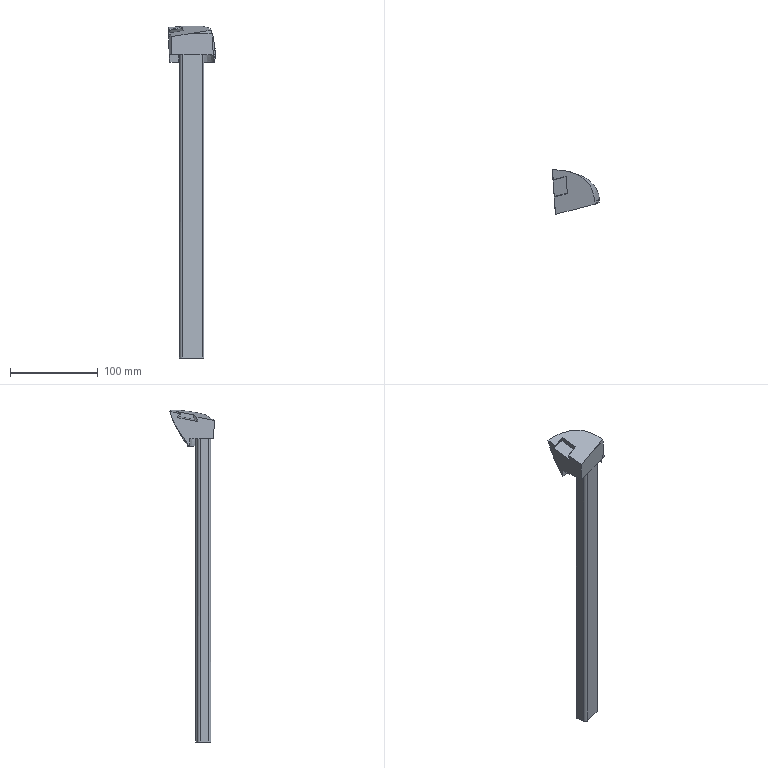Part | STEP file | 车灯-后视镜_id462_x_t | 1 solid | 103 faces | box 53.642 x 50.81 x 378.343 mm | volume 173095 mm3 | spline 63 | plane 24 | cylinder 12 | other 2 | cone 2 | commonest cylinder face diameters 6 x6 1 x4 5.1 x2